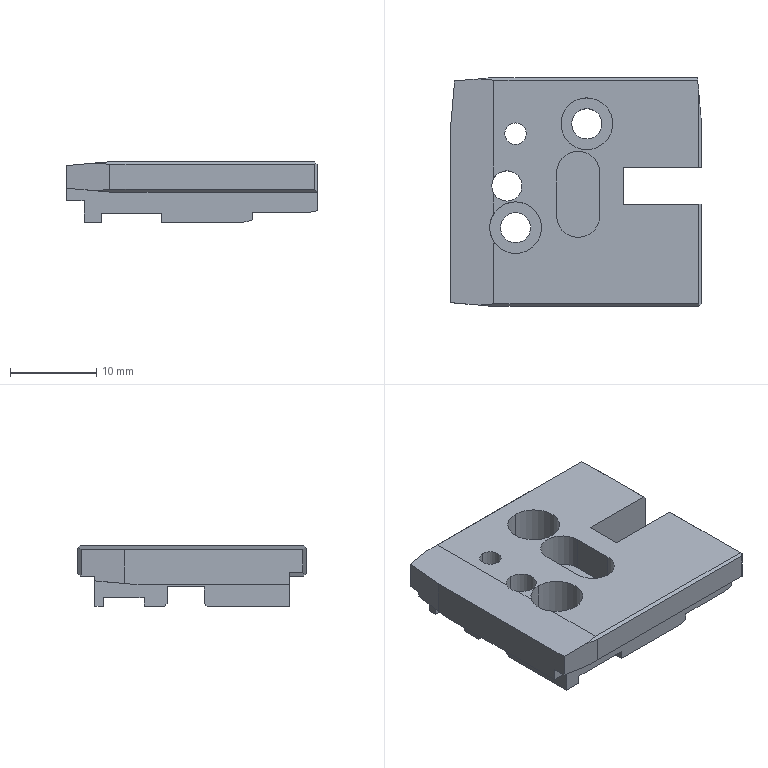Part | NX | 1 solid | 92 faces | box 29 x 26.5 x 7 mm | volume 3482 mm3 | plane 74 | cylinder 18 | commonest cylinder face diameters 3.5 x6 0.8 x4 6 x4 2.5 x2 5 x2